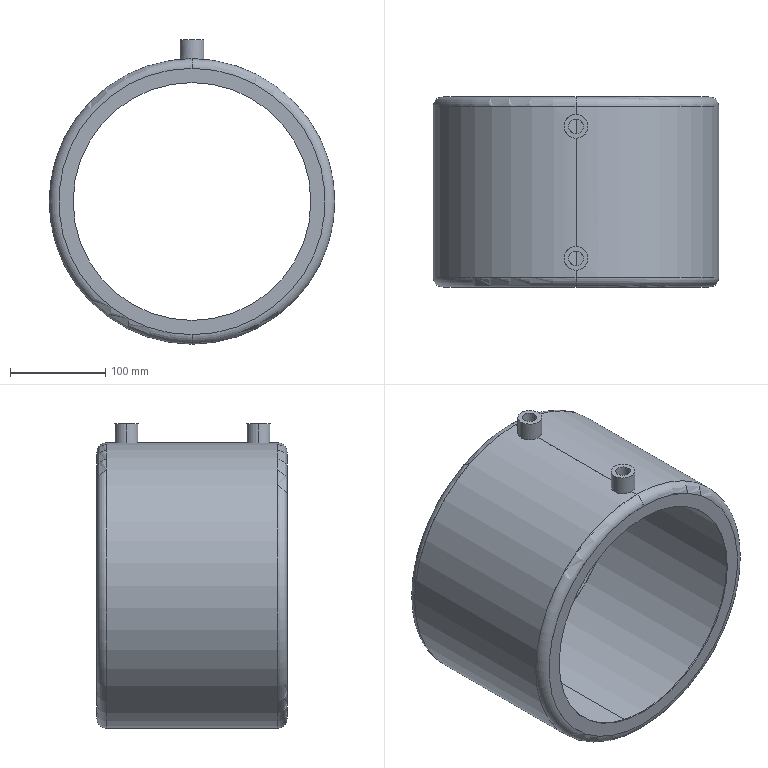Part | SolidWorks | features ICE 2, 3DProfileFeature 1, Extrusion 1, Fillet 1, HoleWzd 1, Shell 1 | 1 solid | 30 faces | box 300 x 200 x 320 mm | volume 277240 mm3 | cylinder 16 | torus 8 | plane 6 | commonest cylinder face diameters 15.25 x4 25 x4 250 x4 297.6 x2 300 x2
STEP:
#1=CARTESIAN_POINT('',(0.,22.375,148.8));
#2=VERTEX_POINT('',#1);
#3=CARTESIAN_POINT('',(-7.625,30.,148.605));
#4=VERTEX_POINT('',#3);
#5=CARTESIAN_POINT('',(0.,22.375,148.8));
#6=CARTESIAN_POINT('',(-0.4973,22.375,148.8));
#7=CARTESIAN_POINT('',(-1.002,22.425,148.797));
#8=CARTESIAN_POINT('',(-1.98,22.62,148.788));
#9=CARTESIAN_POINT('',(-2.455,22.764,148.78));
#10=CARTESIAN_POINT('',(-3.148,23.051,148.767));
#11=CARTESIAN_POINT('',(-3.376,23.159,148.762));
#12=CARTESIAN_POINT('',(-3.818,23.395,148.751));
#13=CARTESIAN_POINT('',(-4.031,23.523,148.746));
#14=CARTESIAN_POINT('',(-4.651,23.937,148.728));
#15=CARTESIAN_POINT('',(-5.036,24.252,148.715));
#16=CARTESIAN_POINT('',(-5.747,24.964,148.689));
#17=CARTESIAN_POINT('',(-6.063,25.35,148.677));
#18=CARTESIAN_POINT('',(-6.477,25.969,148.659));
#19=CARTESIAN_POINT('',(-6.605,26.182,148.653));
#20=CARTESIAN_POINT('',(-6.841,26.623,148.643));
#21=CARTESIAN_POINT('',(-6.949,26.852,148.638));
#22=CARTESIAN_POINT('',(-7.236,27.545,148.624));
#23=CARTESIAN_POINT('',(-7.38,28.02,148.617));
#24=CARTESIAN_POINT('',(-7.575,28.997,148.607));
#25=CARTESIAN_POINT('',(-7.625,29.502,148.605));
#26=CARTESIAN_POINT('',(-7.625,30.,148.605));
#27=B_SPLINE_CURVE_WITH_KNOTS('',3,(#5,#6,#7,#8,#9,#10,#11,#12,#13,#14,#15,#16,#17,#18,#19,#20,#21,#22,#23,#24,#25,#26),.UNSPECIFIED.,.F.,.F.,(4,2,2,2,2,2,2,2,2,2,4),(0.01192,0.01341,0.0149,0.01565,0.01639,0.01788,0.01937,0.02012,0.02086,0.02235,0.02384),.UNSPECIFIED.);
#28=EDGE_CURVE('',#2,#4,#27,.T.);
#29=ORIENTED_EDGE('',*,*,#28,.T.);
#30=CARTESIAN_POINT('',(-7.625,30.,170.));
#31=VERTEX_POINT('',#30);
#32=CARTESIAN_POINT('',(-7.625,30.,170.));
#33=DIRECTION('',(0.,0.,1.));
#34=VECTOR('',#33,1000.);
#35=LINE('',#32,#34);
#36=EDGE_CURVE('',#4,#31,#35,.T.);
#37=ORIENTED_EDGE('',*,*,#36,.T.);
#38=CARTESIAN_POINT('',(7.625,30.,170.));
#39=VERTEX_POINT('',#38);
#40=CARTESIAN_POINT('',(0.,30.,170.));
#41=DIRECTION('',(0.,0.,1.));
#42=DIRECTION('',(1.,0.,0.));
#43=AXIS2_PLACEMENT_3D('',#40,#41,#42);
#44=CIRCLE('',#43,7.625);
#45=EDGE_CURVE('',#31,#39,#44,.T.);
#46=ORIENTED_EDGE('',*,*,#45,.T.);
#47=CARTESIAN_POINT('',(7.625,30.,148.605));
#48=VERTEX_POINT('',#47);
#49=CARTESIAN_POINT('',(7.625,30.,170.));
#50=DIRECTION('',(0.,0.,1.));
#51=VECTOR('',#50,1000.);
#52=LINE('',#49,#51);
#53=EDGE_CURVE('',#48,#39,#52,.T.);
#54=ORIENTED_EDGE('',*,*,#53,.F.);
#55=CARTESIAN_POINT('',(7.625,30.,148.605));
#56=CARTESIAN_POINT('',(7.625,29.496,148.605));
#57=CARTESIAN_POINT('',(7.576,29.,148.607));
#58=CARTESIAN_POINT('',(7.43,28.269,148.614));
#59=CARTESIAN_POINT('',(7.37,28.028,148.617));
#60=CARTESIAN_POINT('',(7.224,27.548,148.625));
#61=CARTESIAN_POINT('',(7.139,27.31,148.629));
#62=CARTESIAN_POINT('',(6.852,26.617,148.642));
#63=CARTESIAN_POINT('',(6.618,26.179,148.653));
#64=CARTESIAN_POINT('',(6.064,25.35,148.677));
#65=CARTESIAN_POINT('',(5.742,24.958,148.69));
#66=CARTESIAN_POINT('',(5.038,24.255,148.715));
#67=CARTESIAN_POINT('',(4.654,23.939,148.728));
#68=CARTESIAN_POINT('',(4.028,23.521,148.746));
#69=CARTESIAN_POINT('',(3.812,23.391,148.751));
#70=CARTESIAN_POINT('',(3.371,23.156,148.762));
#71=CARTESIAN_POINT('',(2.922,22.944,148.772));
#72=CARTESIAN_POINT('',(2.453,22.776,148.78));
#73=CARTESIAN_POINT('',(1.976,22.631,148.787));
#74=CARTESIAN_POINT('',(1.731,22.57,148.79));
#75=CARTESIAN_POINT('',(0.9925,22.423,148.798));
#76=CARTESIAN_POINT('',(0.4975,22.375,148.8));
#77=CARTESIAN_POINT('',(0.,22.375,148.8));
#78=B_SPLINE_CURVE_WITH_KNOTS('',3,(#55,#56,#57,#58,#59,#60,#61,#62,#63,#64,#65,#66,#67,#68,#69,#70,#71,#72,#73,#74,#75,#76,#77),.UNSPECIFIED.,.F.,.F.,(4,2,2,2,2,2,2,2,1,2,2,4),(0.,0.001491,0.002236,0.002981,0.004472,0.005962,0.007453,0.008198,0.008943,0.009688,0.01043,0.01192),.UNSPECIFIED.);
#79=EDGE_CURVE('',#48,#2,#78,.T.);
#80=ORIENTED_EDGE('',*,*,#79,.T.);
#81=EDGE_LOOP('',(#29,#37,#46,#54,#80));
#82=FACE_OUTER_BOUND('',#81,.T.);
#83=CARTESIAN_POINT('',(0.,30.,170.));
#84=DIRECTION('',(0.,0.,1.));
#85=DIRECTION('',(1.,0.,0.));
#86=AXIS2_PLACEMENT_3D('',#83,#84,#85);
#87=CYLINDRICAL_SURFACE('',#86,7.625);
#88=ADVANCED_FACE('',(#82),#87,.F.);
#89=CARTESIAN_POINT('',(0.,161.175,148.8));
#90=VERTEX_POINT('',#89);
#91=CARTESIAN_POINT('',(-7.625,168.8,148.605));
#92=VERTEX_POINT('',#91);
#93=CARTESIAN_POINT('',(0.,161.175,148.8));
#94=CARTESIAN_POINT('',(-0.4973,161.175,148.8));
#95=CARTESIAN_POINT('',(-1.002,161.225,148.797));
#96=CARTESIAN_POINT('',(-1.98,161.42,148.788));
#97=CARTESIAN_POINT('',(-2.455,161.564,148.78));
#98=CARTESIAN_POINT('',(-3.148,161.851,148.767));
#99=CARTESIAN_POINT('',(-3.376,161.959,148.762));
#100=CARTESIAN_POINT('',(-3.818,162.195,148.751));
#101=CARTESIAN_POINT('',(-4.031,162.323,148.746));
#102=CARTESIAN_POINT('',(-4.651,162.737,148.728));
#103=CARTESIAN_POINT('',(-5.036,163.052,148.715));
#104=CARTESIAN_POINT('',(-5.747,163.764,148.689));
#105=CARTESIAN_POINT('',(-6.063,164.15,148.677));
#106=CARTESIAN_POINT('',(-6.477,164.769,148.659));
#107=CARTESIAN_POINT('',(-6.605,164.982,148.653));
#108=CARTESIAN_POINT('',(-6.841,165.423,148.643));
#109=CARTESIAN_POINT('',(-6.949,165.652,148.638));
#110=CARTESIAN_POINT('',(-7.236,166.345,148.624));
#111=CARTESIAN_POINT('',(-7.38,166.82,148.617));
#112=CARTESIAN_POINT('',(-7.575,167.797,148.607));
#113=CARTESIAN_POINT('',(-7.625,168.302,148.605));
#114=CARTESIAN_POINT('',(-7.625,168.8,148.605));
#115=B_SPLINE_CURVE_WITH_KNOTS('',3,(#93,#94,#95,#96,#97,#98,#99,#100,#101,#102,#103,#104,#105,#106,#107,#108,#109,#110,#111,#112,#113,#114),.UNSPECIFIED.,.F.,.F.,(4,2,2,2,2,2,2,2,2,2,4),(0.01192,0.01341,0.0149,0.01565,0.01639,0.01788,0.01937,0.02012,0.02086,0.02235,0.02384),.UNSPECIFIED.);
#116=EDGE_CURVE('',#90,#92,#115,.T.);
#117=ORIENTED_EDGE('',*,*,#116,.T.);
#118=CARTESIAN_POINT('',(-7.625,168.8,170.));
#119=VERTEX_POINT('',#118);
#120=CARTESIAN_POINT('',(-7.625,168.8,170.));
#121=DIRECTION('',(0.,0.,1.));
#122=VECTOR('',#121,1000.);
#123=LINE('',#120,#122);
#124=EDGE_CURVE('',#92,#119,#123,.T.);
#125=ORIENTED_EDGE('',*,*,#124,.T.);
#126=CARTESIAN_POINT('',(7.625,168.8,170.));
#127=VERTEX_POINT('',#126);
#128=CARTESIAN_POINT('',(0.,168.8,170.));
#129=DIRECTION('',(0.,0.,1.));
#130=DIRECTION('',(1.,0.,0.));
#131=AXIS2_PLACEMENT_3D('',#128,#129,#130);
#132=CIRCLE('',#131,7.625);
#133=EDGE_CURVE('',#119,#127,#132,.T.);
#134=ORIENTED_EDGE('',*,*,#133,.T.);
#135=CARTESIAN_POINT('',(7.625,168.8,148.605));
#136=VERTEX_POINT('',#135);
#137=CARTESIAN_POINT('',(7.625,168.8,170.));
#138=DIRECTION('',(0.,0.,1.));
#139=VECTOR('',#138,1000.);
#140=LINE('',#137,#139);
#141=EDGE_CURVE('',#136,#127,#140,.T.);
#142=ORIENTED_EDGE('',*,*,#141,.F.);
#143=CARTESIAN_POINT('',(7.625,168.8,148.605));
#144=CARTESIAN_POINT('',(7.625,168.296,148.605));
#145=CARTESIAN_POINT('',(7.576,167.8,148.607));
#146=CARTESIAN_POINT('',(7.43,167.069,148.614));
#147=CARTESIAN_POINT('',(7.37,166.828,148.617));
#148=CARTESIAN_POINT('',(7.224,166.348,148.625));
#149=CARTESIAN_POINT('',(7.139,166.11,148.629));
#150=CARTESIAN_POINT('',(6.852,165.417,148.642));
#151=CARTESIAN_POINT('',(6.618,164.979,148.653));
#152=CARTESIAN_POINT('',(6.064,164.15,148.677));
#153=CARTESIAN_POINT('',(5.742,163.758,148.69));
#154=CARTESIAN_POINT('',(5.038,163.055,148.715));
#155=CARTESIAN_POINT('',(4.654,162.739,148.728));
#156=CARTESIAN_POINT('',(4.028,162.321,148.746));
#157=CARTESIAN_POINT('',(3.812,162.191,148.751));
#158=CARTESIAN_POINT('',(3.371,161.956,148.762));
#159=CARTESIAN_POINT('',(2.922,161.744,148.772));
#160=CARTESIAN_POINT('',(2.453,161.576,148.78));
#161=CARTESIAN_POINT('',(1.976,161.431,148.787));
#162=CARTESIAN_POINT('',(1.731,161.37,148.79));
#163=CARTESIAN_POINT('',(0.9925,161.223,148.798));
#164=CARTESIAN_POINT('',(0.4975,161.175,148.8));
#165=CARTESIAN_POINT('',(0.,161.175,148.8));
#166=B_SPLINE_CURVE_WITH_KNOTS('',3,(#143,#144,#145,#146,#147,#148,#149,#150,#151,#152,#153,#154,#155,#156,#157,#158,#159,#160,#161,#162,#163,#164,#165),.UNSPECIFIED.,.F.,.F.,(4,2,2,2,2,2,2,2,1,2,2,4),(0.,0.001491,0.002236,0.002981,0.004472,0.005962,0.007453,0.008198,0.008943,0.009688,0.01043,0.01192),.UNSPECIFIED.);
#167=EDGE_CURVE('',#136,#90,#166,.T.);
#168=ORIENTED_EDGE('',*,*,#167,.T.);
#169=EDGE_LOOP('',(#117,#125,#134,#142,#168));
#170=FACE_OUTER_BOUND('',#169,.T.);
#171=CARTESIAN_POINT('',(0.,168.8,170.));
#172=DIRECTION('',(0.,0.,1.));
#173=DIRECTION('',(1.,0.,0.));
#174=AXIS2_PLACEMENT_3D('',#171,#172,#173);
#175=CYLINDRICAL_SURFACE('',#174,7.625);
#176=ADVANCED_FACE('',(#170),#175,.F.);
#177=CARTESIAN_POINT('',(-12.5,168.8,149.478));
#178=VERTEX_POINT('',#177);
#179=CARTESIAN_POINT('',(0.,181.3,150.));
#180=VERTEX_POINT('',#179);
#181=CARTESIAN_POINT('',(-12.5,168.8,149.478));
#182=CARTESIAN_POINT('',(-12.5,169.616,149.478));
#183=CARTESIAN_POINT('',(-12.421,170.428,149.485));
#184=CARTESIAN_POINT('',(-12.181,171.638,149.505));
#185=CARTESIAN_POINT('',(-12.08,172.039,149.513));
#186=CARTESIAN_POINT('',(-11.842,172.823,149.532));
#187=CARTESIAN_POINT('',(-11.567,173.591,149.554));
#188=CARTESIAN_POINT('',(-11.219,174.328,149.58));
#189=CARTESIAN_POINT('',(-10.833,175.049,149.608));
#190=CARTESIAN_POINT('',(-10.621,175.404,149.624));
#191=CARTESIAN_POINT('',(-9.935,176.43,149.671));
#192=CARTESIAN_POINT('',(-9.418,177.06,149.705));
#193=CARTESIAN_POINT('',(-8.553,177.924,149.756));
#194=CARTESIAN_POINT('',(-8.25,178.199,149.773));
#195=CARTESIAN_POINT('',(-7.614,178.722,149.807));
#196=CARTESIAN_POINT('',(-7.282,178.968,149.823));
#197=CARTESIAN_POINT('',(-6.263,179.649,149.871));
#198=CARTESIAN_POINT('',(-5.545,180.033,149.899));
#199=CARTESIAN_POINT('',(-4.41,180.503,149.936));
#200=CARTESIAN_POINT('',(-4.02,180.643,149.947));
#201=CARTESIAN_POINT('',(-3.234,180.881,149.966));
#202=CARTESIAN_POINT('',(-2.837,180.981,149.974));
#203=CARTESIAN_POINT('',(-1.638,181.219,149.993));
#204=CARTESIAN_POINT('',(-0.8258,181.3,150.));
#205=CARTESIAN_POINT('',(0.,181.3,150.));
#206=B_SPLINE_CURVE_WITH_KNOTS('',3,(#181,#182,#183,#184,#185,#186,#187,#188,#189,#190,#191,#192,#193,#194,#195,#196,#197,#198,#199,#200,#201,#202,#203,#204,#205),.UNSPECIFIED.,.F.,.F.,(4,2,2,1,2,2,2,2,2,2,2,2,4),(0.0391,0.04154,0.04276,0.04399,0.04521,0.04643,0.04887,0.0501,0.05132,0.05376,0.05499,0.05621,0.05865),.UNSPECIFIED.);
#207=EDGE_CURVE('',#178,#180,#206,.T.);
#208=ORIENTED_EDGE('',*,*,#207,.F.);
#209=CARTESIAN_POINT('',(-12.5,168.8,170.));
#210=VERTEX_POINT('',#209);
#211=CARTESIAN_POINT('',(-12.5,168.8,-150.001));
#212=DIRECTION('',(0.,0.,1.));
#213=VECTOR('',#212,1000.);
#214=LINE('',#211,#213);
#215=EDGE_CURVE('',#178,#210,#214,.T.);
#216=ORIENTED_EDGE('',*,*,#215,.T.);
#217=CARTESIAN_POINT('',(12.5,168.8,170.));
#218=VERTEX_POINT('',#217);
#219=CARTESIAN_POINT('',(0.,168.8,170.));
#220=DIRECTION('',(0.,0.,1.));
#221=DIRECTION('',(1.,0.,0.));
#222=AXIS2_PLACEMENT_3D('',#219,#220,#221);
#223=CIRCLE('',#222,12.5);
#224=EDGE_CURVE('',#218,#210,#223,.T.);
#225=ORIENTED_EDGE('',*,*,#224,.F.);
#226=CARTESIAN_POINT('',(12.5,168.8,149.478));
#227=VERTEX_POINT('',#226);
#228=CARTESIAN_POINT('',(12.5,168.8,-150.001));
#229=DIRECTION('',(0.,0.,1.));
#230=VECTOR('',#229,1000.);
#231=LINE('',#228,#230);
#232=EDGE_CURVE('',#227,#218,#231,.T.);
#233=ORIENTED_EDGE('',*,*,#232,.F.);
#234=CARTESIAN_POINT('',(0.,181.3,150.));
#235=CARTESIAN_POINT('',(0.8249,181.3,150.));
#236=CARTESIAN_POINT('',(1.639,181.219,149.993));
#237=CARTESIAN_POINT('',(2.836,180.981,149.974));
#238=CARTESIAN_POINT('',(3.232,180.882,149.966));
#239=CARTESIAN_POINT('',(4.016,180.644,149.947));
#240=CARTESIAN_POINT('',(4.407,180.505,149.936));
#241=CARTESIAN_POINT('',(5.542,180.034,149.9));
#242=CARTESIAN_POINT('',(6.259,179.651,149.871));
#243=CARTESIAN_POINT('',(7.278,178.971,149.824));
#244=CARTESIAN_POINT('',(7.608,178.727,149.807));
#245=CARTESIAN_POINT('',(8.245,178.204,149.774));
#246=CARTESIAN_POINT('',(8.548,177.93,149.757));
#247=CARTESIAN_POINT('',(9.412,177.066,149.706));
#248=CARTESIAN_POINT('',(9.93,176.437,149.672));
#249=CARTESIAN_POINT('',(10.615,175.414,149.624));
#250=CARTESIAN_POINT('',(10.828,175.06,149.609));
#251=CARTESIAN_POINT('',(11.214,174.338,149.58));
#252=CARTESIAN_POINT('',(11.562,173.602,149.554));
#253=CARTESIAN_POINT('',(11.838,172.836,149.532));
#254=CARTESIAN_POINT('',(12.076,172.054,149.513));
#255=CARTESIAN_POINT('',(12.177,171.654,149.505));
#256=CARTESIAN_POINT('',(12.419,170.442,149.485));
#257=CARTESIAN_POINT('',(12.5,169.626,149.478));
#258=CARTESIAN_POINT('',(12.5,168.8,149.478));
#259=B_SPLINE_CURVE_WITH_KNOTS('',3,(#234,#235,#236,#237,#238,#239,#240,#241,#242,#243,#244,#245,#246,#247,#248,#249,#250,#251,#252,#253,#254,#255,#256,#257,#258),.UNSPECIFIED.,.F.,.F.,(4,2,2,2,2,2,2,2,2,1,2,2,4),(0.05865,0.06109,0.06231,0.06354,0.06598,0.0672,0.06842,0.07086,0.07208,0.0733,0.07452,0.07574,0.07819),.UNSPECIFIED.);
#260=EDGE_CURVE('',#180,#227,#259,.T.);
#261=ORIENTED_EDGE('',*,*,#260,.F.);
#262=EDGE_LOOP('',(#208,#216,#225,#233,#261));
#263=FACE_OUTER_BOUND('',#262,.T.);
#264=CARTESIAN_POINT('',(0.,168.8,-150.001));
#265=DIRECTION('',(0.,0.,1.));
#266=DIRECTION('',(1.,0.,0.));
#267=AXIS2_PLACEMENT_3D('',#264,#265,#266);
#268=CYLINDRICAL_SURFACE('',#267,12.5);
#269=ADVANCED_FACE('',(#263),#268,.T.);
#270=CARTESIAN_POINT('',(-12.5,30.,149.478));
#271=VERTEX_POINT('',#270);
#272=CARTESIAN_POINT('',(0.,42.5,150.));
#273=VERTEX_POINT('',#272);
#274=CARTESIAN_POINT('',(-12.5,30.,149.478));
#275=CARTESIAN_POINT('',(-12.5,30.816,149.478));
#276=CARTESIAN_POINT('',(-12.421,31.628,149.485));
#277=CARTESIAN_POINT('',(-12.181,32.838,149.505));
#278=CARTESIAN_POINT('',(-12.08,33.239,149.513));
#279=CARTESIAN_POINT('',(-11.842,34.023,149.532));
#280=CARTESIAN_POINT('',(-11.567,34.791,149.554));
#281=CARTESIAN_POINT('',(-11.219,35.528,149.58));
#282=CARTESIAN_POINT('',(-10.833,36.249,149.608));
#283=CARTESIAN_POINT('',(-10.621,36.604,149.624));
#284=CARTESIAN_POINT('',(-9.935,37.63,149.671));
#285=CARTESIAN_POINT('',(-9.418,38.26,149.705));
#286=CARTESIAN_POINT('',(-8.553,39.124,149.756));
#287=CARTESIAN_POINT('',(-8.25,39.399,149.773));
#288=CARTESIAN_POINT('',(-7.614,39.922,149.807));
#289=CARTESIAN_POINT('',(-7.282,40.168,149.823));
#290=CARTESIAN_POINT('',(-6.263,40.849,149.871));
#291=CARTESIAN_POINT('',(-5.545,41.233,149.899));
#292=CARTESIAN_POINT('',(-4.41,41.703,149.936));
#293=CARTESIAN_POINT('',(-4.02,41.843,149.947));
#294=CARTESIAN_POINT('',(-3.234,42.081,149.966));
#295=CARTESIAN_POINT('',(-2.837,42.181,149.974));
#296=CARTESIAN_POINT('',(-1.638,42.419,149.993));
#297=CARTESIAN_POINT('',(-0.8258,42.5,150.));
#298=CARTESIAN_POINT('',(0.,42.5,150.));
#299=B_SPLINE_CURVE_WITH_KNOTS('',3,(#274,#275,#276,#277,#278,#279,#280,#281,#282,#283,#284,#285,#286,#287,#288,#289,#290,#291,#292,#293,#294,#295,#296,#297,#298),.UNSPECIFIED.,.F.,.F.,(4,2,2,1,2,2,2,2,2,2,2,2,4),(0.0391,0.04154,0.04276,0.04399,0.04521,0.04643,0.04887,0.0501,0.05132,0.05376,0.05499,0.05621,0.05865),.UNSPECIFIED.);
#300=EDGE_CURVE('',#271,#273,#299,.T.);
#301=ORIENTED_EDGE('',*,*,#300,.F.);
#302=CARTESIAN_POINT('',(-12.5,30.,170.));
#303=VERTEX_POINT('',#302);
#304=CARTESIAN_POINT('',(-12.5,30.,-150.001));
#305=DIRECTION('',(0.,0.,1.));
#306=VECTOR('',#305,1000.);
#307=LINE('',#304,#306);
#308=EDGE_CURVE('',#271,#303,#307,.T.);
#309=ORIENTED_EDGE('',*,*,#308,.T.);
#310=CARTESIAN_POINT('',(12.5,30.,170.));
#311=VERTEX_POINT('',#310);
#312=CARTESIAN_POINT('',(0.,30.,170.));
#313=DIRECTION('',(0.,0.,1.));
#314=DIRECTION('',(1.,0.,0.));
#315=AXIS2_PLACEMENT_3D('',#312,#313,#314);
#316=CIRCLE('',#315,12.5);
#317=EDGE_CURVE('',#311,#303,#316,.T.);
#318=ORIENTED_EDGE('',*,*,#317,.F.);
#319=CARTESIAN_POINT('',(12.5,30.,149.478));
#320=VERTEX_POINT('',#319);
#321=CARTESIAN_POINT('',(12.5,30.,-150.001));
#322=DIRECTION('',(0.,0.,1.));
#323=VECTOR('',#322,1000.);
#324=LINE('',#321,#323);
#325=EDGE_CURVE('',#320,#311,#324,.T.);
#326=ORIENTED_EDGE('',*,*,#325,.F.);
#327=CARTESIAN_POINT('',(0.,42.5,150.));
#328=CARTESIAN_POINT('',(0.8249,42.5,150.));
#329=CARTESIAN_POINT('',(1.639,42.419,149.993));
#330=CARTESIAN_POINT('',(2.836,42.181,149.974));
#331=CARTESIAN_POINT('',(3.232,42.082,149.966));
#332=CARTESIAN_POINT('',(4.016,41.844,149.947));
#333=CARTESIAN_POINT('',(4.407,41.705,149.936));
#334=CARTESIAN_POINT('',(5.542,41.234,149.9));
#335=CARTESIAN_POINT('',(6.259,40.851,149.871));
#336=CARTESIAN_POINT('',(7.278,40.171,149.824));
#337=CARTESIAN_POINT('',(7.608,39.927,149.807));
#338=CARTESIAN_POINT('',(8.245,39.404,149.774));
#339=CARTESIAN_POINT('',(8.548,39.13,149.757));
#340=CARTESIAN_POINT('',(9.412,38.266,149.706));
#341=CARTESIAN_POINT('',(9.93,37.637,149.672));
#342=CARTESIAN_POINT('',(10.615,36.614,149.624));
#343=CARTESIAN_POINT('',(10.828,36.26,149.609));
#344=CARTESIAN_POINT('',(11.214,35.538,149.58));
#345=CARTESIAN_POINT('',(11.562,34.802,149.554));
#346=CARTESIAN_POINT('',(11.838,34.036,149.532));
#347=CARTESIAN_POINT('',(12.076,33.254,149.513));
#348=CARTESIAN_POINT('',(12.177,32.854,149.505));
#349=CARTESIAN_POINT('',(12.419,31.642,149.485));
#350=CARTESIAN_POINT('',(12.5,30.826,149.478));
#351=CARTESIAN_POINT('',(12.5,30.,149.478));
#352=B_SPLINE_CURVE_WITH_KNOTS('',3,(#327,#328,#329,#330,#331,#332,#333,#334,#335,#336,#337,#338,#339,#340,#341,#342,#343,#344,#345,#346,#347,#348,#349,#350,#351),.UNSPECIFIED.,.F.,.F.,(4,2,2,2,2,2,2,2,2,1,2,2,4),(0.05865,0.06109,0.06231,0.06354,0.06598,0.0672,0.06842,0.07086,0.07208,0.0733,0.07452,0.07574,0.07819),.UNSPECIFIED.);
#353=EDGE_CURVE('',#273,#320,#352,.T.);
#354=ORIENTED_EDGE('',*,*,#353,.F.);
#355=EDGE_LOOP('',(#301,#309,#318,#326,#354));
#356=FACE_OUTER_BOUND('',#355,.T.);
#357=CARTESIAN_POINT('',(0.,30.,-150.001));
#358=DIRECTION('',(0.,0.,1.));
#359=DIRECTION('',(1.,0.,0.));
#360=AXIS2_PLACEMENT_3D('',#357,#358,#359);
#361=CYLINDRICAL_SURFACE('',#360,12.5);
#362=ADVANCED_FACE('',(#356),#361,.T.);
#363=CARTESIAN_POINT('',(0.,190.,148.8));
#364=VERTEX_POINT('',#363);
#365=CARTESIAN_POINT('',(0.,190.,-148.8));
#366=VERTEX_POINT('',#365);
#367=CARTESIAN_POINT('',(0.,190.,0.));
#368=DIRECTION('',(0.,-1.,0.));
#369=DIRECTION('',(0.,0.,-1.));
#370=AXIS2_PLACEMENT_3D('',#367,#368,#369);
#371=CIRCLE('',#370,148.8);
#372=EDGE_CURVE('',#364,#366,#371,.T.);
#373=ORIENTED_EDGE('',*,*,#372,.T.);
#374=CARTESIAN_POINT('',(0.,198.8,-140.));
#375=VERTEX_POINT('',#374);
#376=CARTESIAN_POINT('',(0.,190.,-140.));
#377=DIRECTION('',(1.,0.,0.));
#378=DIRECTION('',(0.,0.,-1.));
#379=AXIS2_PLACEMENT_3D('',#376,#377,#378);
#380=CIRCLE('',#379,8.8);
#381=EDGE_CURVE('',#366,#375,#380,.T.);
#382=ORIENTED_EDGE('',*,*,#381,.T.);
#383=CARTESIAN_POINT('',(0.,198.8,140.));
#384=VERTEX_POINT('',#383);
#385=CARTESIAN_POINT('',(0.,198.8,0.));
#386=DIRECTION('',(0.,1.,0.));
#387=DIRECTION('',(0.,0.,1.));
#388=AXIS2_PLACEMENT_3D('',#385,#386,#387);
#389=CIRCLE('',#388,140.);
#390=EDGE_CURVE('',#375,#384,#389,.T.);
#391=ORIENTED_EDGE('',*,*,#390,.T.);
#392=CARTESIAN_POINT('',(0.,190.,140.));
#393=DIRECTION('',(-1.,0.,0.));
#394=DIRECTION('',(0.,0.,1.));
#395=AXIS2_PLACEMENT_3D('',#392,#393,#394);
#396=CIRCLE('',#395,8.8);
#397=EDGE_CURVE('',#364,#384,#396,.T.);
#398=ORIENTED_EDGE('',*,*,#397,.F.);
#399=EDGE_LOOP('',(#373,#382,#391,#398));
#400=FACE_OUTER_BOUND('',#399,.T.);
#401=CARTESIAN_POINT('',(0.,190.,0.));
#402=DIRECTION('',(0.,1.,0.));
#403=DIRECTION('',(0.,0.,1.));
#404=AXIS2_PLACEMENT_3D('',#401,#402,#403);
#405=TOROIDAL_SURFACE('',#404,140.,8.8);
#406=ADVANCED_FACE('',(#400),#405,.F.);
#407=CARTESIAN_POINT('',(0.,1.2,140.));
#408=VERTEX_POINT('',#407);
#409=CARTESIAN_POINT('',(0.,1.2,-140.));
#410=VERTEX_POINT('',#409);
#411=CARTESIAN_POINT('',(0.,1.2,0.));
#412=DIRECTION('',(0.,-1.,0.));
#413=DIRECTION('',(0.,0.,1.));
#414=AXIS2_PLACEMENT_3D('',#411,#412,#413);
#415=CIRCLE('',#414,140.);
#416=EDGE_CURVE('',#408,#410,#415,.T.);
#417=ORIENTED_EDGE('',*,*,#416,.T.);
#418=CARTESIAN_POINT('',(0.,10.,-148.8));
#419=VERTEX_POINT('',#418);
#420=CARTESIAN_POINT('',(0.,10.,-140.));
#421=DIRECTION('',(1.,0.,0.));
#422=DIRECTION('',(0.,0.,-1.));
#423=AXIS2_PLACEMENT_3D('',#420,#421,#422);
#424=CIRCLE('',#423,8.8);
#425=EDGE_CURVE('',#410,#419,#424,.T.);
#426=ORIENTED_EDGE('',*,*,#425,.T.);
#427=CARTESIAN_POINT('',(0.,10.,148.8));
#428=VERTEX_POINT('',#427);
#429=CARTESIAN_POINT('',(0.,10.,0.));
#430=DIRECTION('',(0.,1.,0.));
#431=DIRECTION('',(0.,0.,-1.));
#432=AXIS2_PLACEMENT_3D('',#429,#430,#431);
#433=CIRCLE('',#432,148.8);
#434=EDGE_CURVE('',#419,#428,#433,.T.);
#435=ORIENTED_EDGE('',*,*,#434,.T.);
#436=CARTESIAN_POINT('',(0.,10.,140.));
#437=DIRECTION('',(-1.,0.,0.));
#438=DIRECTION('',(0.,0.,1.));
#439=AXIS2_PLACEMENT_3D('',#436,#437,#438);
#440=CIRCLE('',#439,8.8);
#441=EDGE_CURVE('',#408,#428,#440,.T.);
#442=ORIENTED_EDGE('',*,*,#441,.F.);
#443=EDGE_LOOP('',(#417,#426,#435,#442));
#444=FACE_OUTER_BOUND('',#443,.T.);
#445=CARTESIAN_POINT('',(0.,10.,0.));
#446=DIRECTION('',(0.,1.,0.));
#447=DIRECTION('',(0.,0.,1.));
#448=AXIS2_PLACEMENT_3D('',#445,#446,#447);
#449=TOROIDAL_SURFACE('',#448,140.,8.8);
#450=ADVANCED_FACE('',(#444),#449,.F.);
#451=ORIENTED_EDGE('',*,*,#372,.F.);
#452=CARTESIAN_POINT('',(0.,176.425,148.8));
#453=VERTEX_POINT('',#452);
#454=CARTESIAN_POINT('',(0.,200.,148.8));
#455=DIRECTION('',(0.,-1.,0.));
#456=VECTOR('',#455,1000.);
#457=LINE('',#454,#456);
#458=EDGE_CURVE('',#364,#453,#457,.T.);
#459=ORIENTED_EDGE('',*,*,#458,.T.);
#460=CARTESIAN_POINT('',(-7.625,168.8,148.605));
#461=CARTESIAN_POINT('',(-7.625,169.298,148.605));
#462=CARTESIAN_POINT('',(-7.577,169.793,148.607));
#463=CARTESIAN_POINT('',(-7.43,170.53,148.614));
#464=CARTESIAN_POINT('',(-7.369,170.776,148.617));
#465=CARTESIAN_POINT('',(-7.224,171.254,148.625));
#466=CARTESIAN_POINT('',(-7.056,171.722,148.633));
#467=CARTESIAN_POINT('',(-6.844,172.172,148.643));
#468=CARTESIAN_POINT('',(-6.609,172.612,148.653));
#469=CARTESIAN_POINT('',(-6.479,172.828,148.659));
#470=CARTESIAN_POINT('',(-6.061,173.454,148.677));
#471=CARTESIAN_POINT('',(-5.745,173.838,148.689));
#472=CARTESIAN_POINT('',(-5.217,174.366,148.709));
#473=CARTESIAN_POINT('',(-5.033,174.534,148.715));
#474=CARTESIAN_POINT('',(-4.645,174.852,148.728));
#475=CARTESIAN_POINT('',(-4.442,175.002,148.734));
#476=CARTESIAN_POINT('',(-3.82,175.418,148.752));
#477=CARTESIAN_POINT('',(-3.382,175.652,148.762));
#478=CARTESIAN_POINT('',(-2.69,175.939,148.776));
#479=CARTESIAN_POINT('',(-2.452,176.024,148.78));
#480=CARTESIAN_POINT('',(-1.972,176.17,148.787));
#481=CARTESIAN_POINT('',(-1.73,176.23,148.79));
#482=CARTESIAN_POINT('',(-0.9986,176.376,148.797));
#483=CARTESIAN_POINT('',(-0.5033,176.425,148.8));
#484=CARTESIAN_POINT('',(0.,176.425,148.8));
#485=B_SPLINE_CURVE_WITH_KNOTS('',3,(#460,#461,#462,#463,#464,#465,#466,#467,#468,#469,#470,#471,#472,#473,#474,#475,#476,#477,#478,#479,#480,#481,#482,#483,#484),.UNSPECIFIED.,.F.,.F.,(4,2,2,1,2,2,2,2,2,2,2,2,4),(0.02384,0.02533,0.02608,0.02682,0.02757,0.02832,0.02981,0.03055,0.0313,0.03279,0.03353,0.03428,0.03577),.UNSPECIFIED.);
#486=EDGE_CURVE('',#92,#453,#485,.T.);
#487=ORIENTED_EDGE('',*,*,#486,.F.);
#488=ORIENTED_EDGE('',*,*,#116,.F.);
#489=CARTESIAN_POINT('',(0.,37.625,148.8));
#490=VERTEX_POINT('',#489);
#491=CARTESIAN_POINT('',(0.,200.,148.8));
#492=DIRECTION('',(0.,-1.,0.));
#493=VECTOR('',#492,1000.);
#494=LINE('',#491,#493);
#495=EDGE_CURVE('',#90,#490,#494,.T.);
#496=ORIENTED_EDGE('',*,*,#495,.T.);
#497=CARTESIAN_POINT('',(-7.625,30.,148.605));
#498=CARTESIAN_POINT('',(-7.625,30.498,148.605));
#499=CARTESIAN_POINT('',(-7.577,30.993,148.607));
#500=CARTESIAN_POINT('',(-7.43,31.73,148.614));
#501=CARTESIAN_POINT('',(-7.369,31.976,148.617));
#502=CARTESIAN_POINT('',(-7.224,32.454,148.625));
#503=CARTESIAN_POINT('',(-7.056,32.922,148.633));
#504=CARTESIAN_POINT('',(-6.844,33.372,148.643));
#505=CARTESIAN_POINT('',(-6.609,33.812,148.653));
#506=CARTESIAN_POINT('',(-6.479,34.028,148.659));
#507=CARTESIAN_POINT('',(-6.061,34.654,148.677));
#508=CARTESIAN_POINT('',(-5.745,35.038,148.689));
#509=CARTESIAN_POINT('',(-5.217,35.566,148.709));
#510=CARTESIAN_POINT('',(-5.033,35.734,148.715));
#511=CARTESIAN_POINT('',(-4.645,36.052,148.728));
#512=CARTESIAN_POINT('',(-4.442,36.202,148.734));
#513=CARTESIAN_POINT('',(-3.82,36.618,148.752));
#514=CARTESIAN_POINT('',(-3.382,36.852,148.762));
#515=CARTESIAN_POINT('',(-2.69,37.139,148.776));
#516=CARTESIAN_POINT('',(-2.452,37.224,148.78));
#517=CARTESIAN_POINT('',(-1.972,37.37,148.787));
#518=CARTESIAN_POINT('',(-1.73,37.43,148.79));
#519=CARTESIAN_POINT('',(-0.9986,37.576,148.797));
#520=CARTESIAN_POINT('',(-0.5033,37.625,148.8));
#521=CARTESIAN_POINT('',(0.,37.625,148.8));
#522=B_SPLINE_CURVE_WITH_KNOTS('',3,(#497,#498,#499,#500,#501,#502,#503,#504,#505,#506,#507,#508,#509,#510,#511,#512,#513,#514,#515,#516,#517,#518,#519,#520,#521),.UNSPECIFIED.,.F.,.F.,(4,2,2,1,2,2,2,2,2,2,2,2,4),(0.02384,0.02533,0.02608,0.02682,0.02757,0.02832,0.02981,0.03055,0.0313,0.03279,0.03353,0.03428,0.03577),.UNSPECIFIED.);
#523=EDGE_CURVE('',#4,#490,#522,.T.);
#524=ORIENTED_EDGE('',*,*,#523,.F.);
#525=ORIENTED_EDGE('',*,*,#28,.F.);
#526=CARTESIAN_POINT('',(0.,200.,148.8));
#527=DIRECTION('',(0.,-1.,0.));
#528=VECTOR('',#527,1000.);
#529=LINE('',#526,#528);
#530=EDGE_CURVE('',#2,#428,#529,.T.);
#531=ORIENTED_EDGE('',*,*,#530,.T.);
#532=ORIENTED_EDGE('',*,*,#434,.F.);
#533=CARTESIAN_POINT('',(0.,200.,-148.8));
#534=DIRECTION('',(0.,-1.,0.));
#535=VECTOR('',#534,1000.);
#536=LINE('',#533,#535);
#537=EDGE_CURVE('',#366,#419,#536,.T.);
#538=ORIENTED_EDGE('',*,*,#537,.F.);
#539=EDGE_LOOP('',(#451,#459,#487,#488,#496,#524,#525,#531,#532,#538));
#540=FACE_OUTER_BOUND('',#539,.T.);
#541=CARTESIAN_POINT('',(0.,200.,0.));
#542=DIRECTION('',(0.,-1.,0.));
#543=DIRECTION('',(0.,0.,-1.));
#544=AXIS2_PLACEMENT_3D('',#541,#542,#543);
#545=CYLINDRICAL_SURFACE('',#544,148.8);
#546=ADVANCED_FACE('',(#540),#545,.F.);
#547=CARTESIAN_POINT('',(0.,0.,-125.));
#548=VERTEX_POINT('',#547);
#549=CARTESIAN_POINT('',(0.,0.,125.));
#550=VERTEX_POINT('',#549);
#551=CARTESIAN_POINT('',(0.,0.,0.));
#552=DIRECTION('',(0.,1.,0.));
#553=DIRECTION('',(0.,0.,1.));
#554=AXIS2_PLACEMENT_3D('',#551,#552,#553);
#555=CIRCLE('',#554,125.);
#556=EDGE_CURVE('',#548,#550,#555,.T.);
#557=ORIENTED_EDGE('',*,*,#556,.F.);
#558=CARTESIAN_POINT('',(0.,1.2,-125.));
#559=VERTEX_POINT('',#558);
#560=CARTESIAN_POINT('',(0.,0.,-125.));
#561=DIRECTION('',(0.,1.,0.));
#562=VECTOR('',#561,1000.);
#563=LINE('',#560,#562);
#564=EDGE_CURVE('',#548,#559,#563,.T.);
#565=ORIENTED_EDGE('',*,*,#564,.T.);
#566=CARTESIAN_POINT('',(0.,1.2,125.));
#567=VERTEX_POINT('',#566);
#568=CARTESIAN_POINT('',(0.,1.2,0.));
#569=DIRECTION('',(0.,1.,0.));
#570=DIRECTION('',(0.,0.,1.));
#571=AXIS2_PLACEMENT_3D('',#568,#569,#570);
#572=CIRCLE('',#571,125.);
#573=EDGE_CURVE('',#559,#567,#572,.T.);
#574=ORIENTED_EDGE('',*,*,#573,.T.);
#575=CARTESIAN_POINT('',(0.,0.,125.));
#576=DIRECTION('',(0.,1.,0.));
#577=VECTOR('',#576,1000.);
#578=LINE('',#575,#577);
#579=EDGE_CURVE('',#550,#567,#578,.T.);
#580=ORIENTED_EDGE('',*,*,#579,.F.);
#581=EDGE_LOOP('',(#557,#565,#574,#580));
#582=FACE_OUTER_BOUND('',#581,.T.);
#583=CARTESIAN_POINT('',(0.,0.,0.));
#584=DIRECTION('',(0.,1.,0.));
#585=DIRECTION('',(0.,0.,1.));
#586=AXIS2_PLACEMENT_3D('',#583,#584,#585);
#587=CYLINDRICAL_SURFACE('',#586,125.);
#588=ADVANCED_FACE('',(#582),#587,.F.);
#589=CARTESIAN_POINT('',(0.,190.,-150.));
#590=VERTEX_POINT('',#589);
#591=CARTESIAN_POINT('',(0.,190.,150.));
#592=VERTEX_POINT('',#591);
#593=CARTESIAN_POINT('',(0.,190.,0.));
#594=DIRECTION('',(0.,-1.,0.));
#595=DIRECTION('',(0.,0.,1.));
#596=AXIS2_PLACEMENT_3D('',#593,#594,#595);
#597=CIRCLE('',#596,150.);
#598=EDGE_CURVE('',#590,#592,#597,.T.);
#599=ORIENTED_EDGE('',*,*,#598,.F.);
#600=CARTESIAN_POINT('',(0.,200.,-140.));
#601=VERTEX_POINT('',#600);
#602=CARTESIAN_POINT('',(0.,190.,-140.));
#603=DIRECTION('',(1.,0.,0.));
#604=DIRECTION('',(0.,0.,-1.));
#605=AXIS2_PLACEMENT_3D('',#602,#603,#604);
#606=CIRCLE('',#605,10.);
#607=EDGE_CURVE('',#590,#601,#606,.T.);
#608=ORIENTED_EDGE('',*,*,#607,.T.);
#609=CARTESIAN_POINT('',(0.,200.,140.));
#610=VERTEX_POINT('',#609);
#611=CARTESIAN_POINT('',(0.,200.,0.));
#612=DIRECTION('',(0.,1.,0.));
#613=DIRECTION('',(0.,0.,1.));
#614=AXIS2_PLACEMENT_3D('',#611,#612,#613);
#615=CIRCLE('',#614,140.);
#616=EDGE_CURVE('',#610,#601,#615,.T.);
#617=ORIENTED_EDGE('',*,*,#616,.F.);
#618=CARTESIAN_POINT('',(0.,190.,140.));
#619=DIRECTION('',(-1.,0.,0.));
#620=DIRECTION('',(0.,0.,1.));
#621=AXIS2_PLACEMENT_3D('',#618,#619,#620);
#622=CIRCLE('',#621,10.);
#623=EDGE_CURVE('',#592,#610,#622,.T.);
#624=ORIENTED_EDGE('',*,*,#623,.F.);
#625=EDGE_LOOP('',(#599,#608,#617,#624));
#626=FACE_OUTER_BOUND('',#625,.T.);
#627=CARTESIAN_POINT('',(0.,190.,0.));
#628=DIRECTION('',(0.,1.,0.));
#629=DIRECTION('',(0.,0.,1.));
#630=AXIS2_PLACEMENT_3D('',#627,#628,#629);
#631=TOROIDAL_SURFACE('',#630,140.,10.);
#632=ADVANCED_FACE('',(#626),#631,.T.);
#633=CARTESIAN_POINT('',(0.,0.,-140.));
#634=VERTEX_POINT('',#633);
#635=CARTESIAN_POINT('',(0.,0.,140.));
#636=VERTEX_POINT('',#635);
#637=CARTESIAN_POINT('',(0.,0.,0.));
#638=DIRECTION('',(0.,-1.,0.));
#639=DIRECTION('',(0.,0.,1.));
#640=AXIS2_PLACEMENT_3D('',#637,#638,#639);
#641=CIRCLE('',#640,140.);
#642=EDGE_CURVE('',#634,#636,#641,.T.);
#643=ORIENTED_EDGE('',*,*,#642,.F.);
#644=CARTESIAN_POINT('',(0.,10.,-150.));
#645=VERTEX_POINT('',#644);
#646=CARTESIAN_POINT('',(0.,10.,-140.));
#647=DIRECTION('',(1.,0.,0.));
#648=DIRECTION('',(0.,0.,-1.));
#649=AXIS2_PLACEMENT_3D('',#646,#647,#648);
#650=CIRCLE('',#649,10.);
#651=EDGE_CURVE('',#634,#645,#650,.T.);
#652=ORIENTED_EDGE('',*,*,#651,.T.);
#653=CARTESIAN_POINT('',(0.,10.,150.));
#654=VERTEX_POINT('',#653);
#655=CARTESIAN_POINT('',(0.,10.,0.));
#656=DIRECTION('',(0.,1.,0.));
#657=DIRECTION('',(0.,0.,1.));
#658=AXIS2_PLACEMENT_3D('',#655,#656,#657);
#659=CIRCLE('',#658,150.);
#660=EDGE_CURVE('',#654,#645,#659,.T.);
#661=ORIENTED_EDGE('',*,*,#660,.F.);
#662=CARTESIAN_POINT('',(0.,10.,140.));
#663=DIRECTION('',(-1.,0.,0.));
#664=DIRECTION('',(0.,0.,1.));
#665=AXIS2_PLACEMENT_3D('',#662,#663,#664);
#666=CIRCLE('',#665,10.);
#667=EDGE_CURVE('',#636,#654,#666,.T.);
#668=ORIENTED_EDGE('',*,*,#667,.F.);
#669=EDGE_LOOP('',(#643,#652,#661,#668));
#670=FACE_OUTER_BOUND('',#669,.T.);
#671=CARTESIAN_POINT('',(0.,10.,0.));
#672=DIRECTION('',(0.,1.,0.));
#673=DIRECTION('',(0.,0.,1.));
#674=AXIS2_PLACEMENT_3D('',#671,#672,#673);
#675=TOROIDAL_SURFACE('',#674,140.,10.);
#676=ADVANCED_FACE('',(#670),#675,.T.);
#677=ORIENTED_EDGE('',*,*,#598,.T.);
#678=CARTESIAN_POINT('',(0.,200.,150.));
#679=DIRECTION('',(0.,-1.,0.));
#680=VECTOR('',#679,1000.);
#681=LINE('',#678,#680);
#682=EDGE_CURVE('',#592,#180,#681,.T.);
#683=ORIENTED_EDGE('',*,*,#682,.T.);
#684=ORIENTED_EDGE('',*,*,#260,.T.);
#685=CARTESIAN_POINT('',(0.,156.3,150.));
#686=VERTEX_POINT('',#685);
#687=CARTESIAN_POINT('',(12.5,168.8,149.478));
#688=CARTESIAN_POINT('',(12.5,167.974,149.478));
#689=CARTESIAN_POINT('',(12.419,167.161,149.485));
#690=CARTESIAN_POINT('',(12.18,165.962,149.505));
#691=CARTESIAN_POINT('',(12.081,165.566,149.513));
#692=CARTESIAN_POINT('',(11.843,164.78,149.532));
#693=CARTESIAN_POINT('',(11.703,164.39,149.543));
#694=CARTESIAN_POINT('',(11.232,163.254,149.579));
#695=CARTESIAN_POINT('',(10.848,162.536,149.608));
#696=CARTESIAN_POINT('',(10.167,161.517,149.655));
#697=CARTESIAN_POINT('',(9.922,161.186,149.672));
#698=CARTESIAN_POINT('',(9.399,160.549,149.705));
#699=CARTESIAN_POINT('',(9.124,160.246,149.723));
#700=CARTESIAN_POINT('',(8.259,159.382,149.774));
#701=CARTESIAN_POINT('',(7.629,158.864,149.807));
#702=CARTESIAN_POINT('',(6.604,158.179,149.855));
#703=CARTESIAN_POINT('',(6.249,157.966,149.87));
#704=CARTESIAN_POINT('',(5.527,157.581,149.899));
#705=CARTESIAN_POINT('',(4.79,157.233,149.925));
#706=CARTESIAN_POINT('',(4.023,156.958,149.947));
#707=CARTESIAN_POINT('',(3.24,156.72,149.966));
#708=CARTESIAN_POINT('',(2.838,156.62,149.974));
#709=CARTESIAN_POINT('',(1.627,156.379,149.993));
#710=CARTESIAN_POINT('',(0.8159,156.3,150.));
#711=CARTESIAN_POINT('',(0.,156.3,150.));
#712=B_SPLINE_CURVE_WITH_KNOTS('',3,(#687,#688,#689,#690,#691,#692,#693,#694,#695,#696,#697,#698,#699,#700,#701,#702,#703,#704,#705,#706,#707,#708,#709,#710,#711),.UNSPECIFIED.,.F.,.F.,(4,2,2,2,2,2,2,2,2,1,2,2,4),(0.,0.002444,0.003666,0.004888,0.007332,0.008555,0.009777,0.01222,0.01344,0.01466,0.01589,0.01711,0.01955),.UNSPECIFIED.);
#713=EDGE_CURVE('',#227,#686,#712,.T.);
#714=ORIENTED_EDGE('',*,*,#713,.T.);
#715=CARTESIAN_POINT('',(0.,200.,150.));
#716=DIRECTION('',(0.,-1.,0.));
#717=VECTOR('',#716,1000.);
#718=LINE('',#715,#717);
#719=EDGE_CURVE('',#686,#273,#718,.T.);
#720=ORIENTED_EDGE('',*,*,#719,.T.);
#721=ORIENTED_EDGE('',*,*,#353,.T.);
#722=CARTESIAN_POINT('',(0.,17.5,150.));
#723=VERTEX_POINT('',#722);
#724=CARTESIAN_POINT('',(12.5,30.,149.478));
#725=CARTESIAN_POINT('',(12.5,29.174,149.478));
#726=CARTESIAN_POINT('',(12.419,28.361,149.485));
#727=CARTESIAN_POINT('',(12.18,27.162,149.505));
#728=CARTESIAN_POINT('',(12.081,26.766,149.513));
#729=CARTESIAN_POINT('',(11.843,25.98,149.532));
#730=CARTESIAN_POINT('',(11.703,25.59,149.543));
#731=CARTESIAN_POINT('',(11.232,24.454,149.579));
#732=CARTESIAN_POINT('',(10.848,23.736,149.608));
#733=CARTESIAN_POINT('',(10.167,22.717,149.655));
#734=CARTESIAN_POINT('',(9.922,22.386,149.672));
#735=CARTESIAN_POINT('',(9.399,21.749,149.705));
#736=CARTESIAN_POINT('',(9.124,21.446,149.723));
#737=CARTESIAN_POINT('',(8.259,20.582,149.774));
#738=CARTESIAN_POINT('',(7.629,20.064,149.807));
#739=CARTESIAN_POINT('',(6.604,19.379,149.855));
#740=CARTESIAN_POINT('',(6.249,19.166,149.87));
#741=CARTESIAN_POINT('',(5.527,18.781,149.899));
#742=CARTESIAN_POINT('',(4.79,18.433,149.925));
#743=CARTESIAN_POINT('',(4.023,18.158,149.947));
#744=CARTESIAN_POINT('',(3.24,17.92,149.966));
#745=CARTESIAN_POINT('',(2.838,17.82,149.974));
#746=CARTESIAN_POINT('',(1.627,17.579,149.993));
#747=CARTESIAN_POINT('',(0.8159,17.5,150.));
#748=CARTESIAN_POINT('',(0.,17.5,150.));
#749=B_SPLINE_CURVE_WITH_KNOTS('',3,(#724,#725,#726,#727,#728,#729,#730,#731,#732,#733,#734,#735,#736,#737,#738,#739,#740,#741,#742,#743,#744,#745,#746,#747,#748),.UNSPECIFIED.,.F.,.F.,(4,2,2,2,2,2,2,2,2,1,2,2,4),(0.,0.002444,0.003666,0.004888,0.007332,0.008555,0.009777,0.01222,0.01344,0.01466,0.01589,0.01711,0.01955),.UNSPECIFIED.);
#750=EDGE_CURVE('',#320,#723,#749,.T.);
#751=ORIENTED_EDGE('',*,*,#750,.T.);
#752=CARTESIAN_POINT('',(0.,200.,150.));
#753=DIRECTION('',(0.,-1.,0.));
#754=VECTOR('',#753,1000.);
#755=LINE('',#752,#754);
#756=EDGE_CURVE('',#723,#654,#755,.T.);
#757=ORIENTED_EDGE('',*,*,#756,.T.);
#758=ORIENTED_EDGE('',*,*,#660,.T.);
#759=CARTESIAN_POINT('',(0.,200.,-150.));
#760=DIRECTION('',(0.,-1.,0.));
#761=VECTOR('',#760,1000.);
#762=LINE('',#759,#761);
#763=EDGE_CURVE('',#590,#645,#762,.T.);
#764=ORIENTED_EDGE('',*,*,#763,.F.);
#765=EDGE_LOOP('',(#677,#683,#684,#714,#720,#721,#751,#757,#758,#764));
#766=FACE_OUTER_BOUND('',#765,.T.);
#767=CARTESIAN_POINT('',(0.,200.,0.));
#768=DIRECTION('',(0.,-1.,0.));
#769=DIRECTION('',(0.,0.,-1.));
#770=AXIS2_PLACEMENT_3D('',#767,#768,#769);
#771=CYLINDRICAL_SURFACE('',#770,150.);
#772=ADVANCED_FACE('',(#766),#771,.T.);
#773=CARTESIAN_POINT('',(0.,198.8,-125.));
#774=VERTEX_POINT('',#773);
#775=CARTESIAN_POINT('',(0.,198.8,125.));
#776=VERTEX_POINT('',#775);
#777=CARTESIAN_POINT('',(0.,198.8,0.));
#778=DIRECTION('',(0.,1.,0.));
#779=DIRECTION('',(0.,0.,1.));
#780=AXIS2_PLACEMENT_3D('',#777,#778,#779);
#781=CIRCLE('',#780,125.);
#782=EDGE_CURVE('',#774,#776,#781,.T.);
#783=ORIENTED_EDGE('',*,*,#782,.F.);
#784=CARTESIAN_POINT('',(0.,200.,-125.));
#785=VERTEX_POINT('',#784);
#786=CARTESIAN_POINT('',(0.,0.,-125.));
#787=DIRECTION('',(0.,1.,0.));
#788=VECTOR('',#787,1000.);
#789=LINE('',#786,#788);
#790=EDGE_CURVE('',#774,#785,#789,.T.);
#791=ORIENTED_EDGE('',*,*,#790,.T.);
#792=CARTESIAN_POINT('',(0.,200.,125.));
#793=VERTEX_POINT('',#792);
#794=CARTESIAN_POINT('',(0.,200.,0.));
#795=DIRECTION('',(0.,1.,0.));
#796=DIRECTION('',(0.,0.,1.));
#797=AXIS2_PLACEMENT_3D('',#794,#795,#796);
#798=CIRCLE('',#797,125.);
#799=EDGE_CURVE('',#785,#793,#798,.T.);
#800=ORIENTED_EDGE('',*,*,#799,.T.);
#801=CARTESIAN_POINT('',(0.,0.,125.));
#802=DIRECTION('',(0.,1.,0.));
#803=VECTOR('',#802,1000.);
#804=LINE('',#801,#803);
#805=EDGE_CURVE('',#776,#793,#804,.T.);
#806=ORIENTED_EDGE('',*,*,#805,.F.);
#807=EDGE_LOOP('',(#783,#791,#800,#806));
#808=FACE_OUTER_BOUND('',#807,.T.);
#809=CARTESIAN_POINT('',(0.,0.,0.));
#810=DIRECTION('',(0.,1.,0.));
#811=DIRECTION('',(0.,0.,1.));
#812=AXIS2_PLACEMENT_3D('',#809,#810,#811);
#813=CYLINDRICAL_SURFACE('',#812,125.);
#814=ADVANCED_FACE('',(#808),#813,.F.);
#815=ORIENTED_EDGE('',*,*,#790,.F.);
#816=CARTESIAN_POINT('',(0.,198.8,0.));
#817=DIRECTION('',(0.,1.,0.));
#818=DIRECTION('',(0.,0.,1.));
#819=AXIS2_PLACEMENT_3D('',#816,#817,#818);
#820=CIRCLE('',#819,125.);
#821=EDGE_CURVE('',#776,#774,#820,.T.);
#822=ORIENTED_EDGE('',*,*,#821,.F.);
#823=ORIENTED_EDGE('',*,*,#805,.T.);
#824=CARTESIAN_POINT('',(0.,200.,0.));
#825=DIRECTION('',(0.,1.,0.));
#826=DIRECTION('',(0.,0.,1.));
#827=AXIS2_PLACEMENT_3D('',#824,#825,#826);
#828=CIRCLE('',#827,125.);
#829=EDGE_CURVE('',#793,#785,#828,.T.);
#830=ORIENTED_EDGE('',*,*,#829,.T.);
#831=EDGE_LOOP('',(#815,#822,#823,#830));
#832=FACE_OUTER_BOUND('',#831,.T.);
#833=CARTESIAN_POINT('',(0.,0.,0.));
#834=DIRECTION('',(0.,1.,0.));
#835=DIRECTION('',(0.,0.,1.));
#836=AXIS2_PLACEMENT_3D('',#833,#834,#835);
#837=CYLINDRICAL_SURFACE('',#836,125.);
#838=ADVANCED_FACE('',(#832),#837,.F.);
#839=ORIENTED_EDGE('',*,*,#682,.F.);
#840=CARTESIAN_POINT('',(0.,190.,0.));
#841=DIRECTION('',(0.,-1.,0.));
#842=DIRECTION('',(0.,0.,1.));
#843=AXIS2_PLACEMENT_3D('',#840,#841,#842);
#844=CIRCLE('',#843,150.);
#845=EDGE_CURVE('',#592,#590,#844,.T.);
#846=ORIENTED_EDGE('',*,*,#845,.T.);
#847=ORIENTED_EDGE('',*,*,#763,.T.);
#848=CARTESIAN_POINT('',(0.,10.,0.));
#849=DIRECTION('',(0.,1.,0.));
#850=DIRECTION('',(0.,0.,1.));
#851=AXIS2_PLACEMENT_3D('',#848,#849,#850);
#852=CIRCLE('',#851,150.);
#853=EDGE_CURVE('',#645,#654,#852,.T.);
#854=ORIENTED_EDGE('',*,*,#853,.T.);
#855=ORIENTED_EDGE('',*,*,#756,.F.);
#856=CARTESIAN_POINT('',(0.,17.5,150.));
#857=CARTESIAN_POINT('',(-0.4078,17.5,150.));
#858=CARTESIAN_POINT('',(-0.8166,17.52,149.998));
#859=CARTESIAN_POINT('',(-1.637,17.601,149.992));
#860=CARTESIAN_POINT('',(-2.045,17.662,149.987));
#861=CARTESIAN_POINT('',(-3.247,17.901,149.967));
#862=CARTESIAN_POINT('',(-4.026,18.138,149.948));
#863=CARTESIAN_POINT('',(-5.161,18.608,149.912));
#864=CARTESIAN_POINT('',(-5.536,18.785,149.898));
#865=CARTESIAN_POINT('',(-6.259,19.172,149.87));
#866=CARTESIAN_POINT('',(-6.609,19.382,149.855));
#867=CARTESIAN_POINT('',(-7.624,20.061,149.808));
#868=CARTESIAN_POINT('',(-8.255,20.578,149.774));
#869=CARTESIAN_POINT('',(-9.422,21.745,149.705));
#870=CARTESIAN_POINT('',(-9.939,22.376,149.671));
#871=CARTESIAN_POINT('',(-10.618,23.391,149.624));
#872=CARTESIAN_POINT('',(-10.828,23.741,149.609));
#873=CARTESIAN_POINT('',(-11.215,24.464,149.58));
#874=CARTESIAN_POINT('',(-11.392,24.839,149.567));
#875=CARTESIAN_POINT('',(-11.862,25.974,149.531));
#876=CARTESIAN_POINT('',(-12.099,26.753,149.511));
#877=CARTESIAN_POINT('',(-12.338,27.955,149.492));
#878=CARTESIAN_POINT('',(-12.399,28.362,149.487));
#879=CARTESIAN_POINT('',(-12.48,29.183,149.48));
#880=CARTESIAN_POINT('',(-12.5,29.592,149.478));
#881=CARTESIAN_POINT('',(-12.5,30.,149.478));
#882=B_SPLINE_CURVE_WITH_KNOTS('',3,(#856,#857,#858,#859,#860,#861,#862,#863,#864,#865,#866,#867,#868,#869,#870,#871,#872,#873,#874,#875,#876,#877,#878,#879,#880,#881),.UNSPECIFIED.,.F.,.F.,(4,2,2,2,2,2,2,2,2,2,2,2,4),(0.01955,0.02077,0.022,0.02444,0.02566,0.02688,0.02933,0.03177,0.03299,0.03421,0.03665,0.03788,0.0391),.UNSPECIFIED.);
#883=EDGE_CURVE('',#723,#271,#882,.T.);
#884=ORIENTED_EDGE('',*,*,#883,.T.);
#885=ORIENTED_EDGE('',*,*,#300,.T.);
#886=ORIENTED_EDGE('',*,*,#719,.F.);
#887=CARTESIAN_POINT('',(0.,156.3,150.));
#888=CARTESIAN_POINT('',(-0.4078,156.3,150.));
#889=CARTESIAN_POINT('',(-0.8166,156.32,149.998));
#890=CARTESIAN_POINT('',(-1.637,156.401,149.992));
#891=CARTESIAN_POINT('',(-2.045,156.462,149.987));
#892=CARTESIAN_POINT('',(-3.247,156.701,149.967));
#893=CARTESIAN_POINT('',(-4.026,156.938,149.948));
#894=CARTESIAN_POINT('',(-5.161,157.408,149.912));
#895=CARTESIAN_POINT('',(-5.536,157.585,149.898));
#896=CARTESIAN_POINT('',(-6.259,157.972,149.87));
#897=CARTESIAN_POINT('',(-6.609,158.182,149.855));
#898=CARTESIAN_POINT('',(-7.624,158.861,149.808));
#899=CARTESIAN_POINT('',(-8.255,159.378,149.774));
#900=CARTESIAN_POINT('',(-9.422,160.545,149.705));
#901=CARTESIAN_POINT('',(-9.939,161.176,149.671));
#902=CARTESIAN_POINT('',(-10.618,162.191,149.624));
#903=CARTESIAN_POINT('',(-10.828,162.541,149.609));
#904=CARTESIAN_POINT('',(-11.215,163.264,149.58));
#905=CARTESIAN_POINT('',(-11.392,163.639,149.567));
#906=CARTESIAN_POINT('',(-11.862,164.774,149.531));
#907=CARTESIAN_POINT('',(-12.099,165.553,149.511));
#908=CARTESIAN_POINT('',(-12.338,166.755,149.492));
#909=CARTESIAN_POINT('',(-12.399,167.162,149.487));
#910=CARTESIAN_POINT('',(-12.48,167.983,149.48));
#911=CARTESIAN_POINT('',(-12.5,168.392,149.478));
#912=CARTESIAN_POINT('',(-12.5,168.8,149.478));
#913=B_SPLINE_CURVE_WITH_KNOTS('',3,(#887,#888,#889,#890,#891,#892,#893,#894,#895,#896,#897,#898,#899,#900,#901,#902,#903,#904,#905,#906,#907,#908,#909,#910,#911,#912),.UNSPECIFIED.,.F.,.F.,(4,2,2,2,2,2,2,2,2,2,2,2,4),(0.01955,0.02077,0.022,0.02444,0.02566,0.02688,0.02933,0.03177,0.03299,0.03421,0.03665,0.03788,0.0391),.UNSPECIFIED.);
#914=EDGE_CURVE('',#686,#178,#913,.T.);
#915=ORIENTED_EDGE('',*,*,#914,.T.);
#916=ORIENTED_EDGE('',*,*,#207,.T.);
#917=EDGE_LOOP('',(#839,#846,#847,#854,#855,#884,#885,#886,#915,#916));
#918=FACE_OUTER_BOUND('',#917,.T.);
#919=CARTESIAN_POINT('',(0.,200.,0.));
#920=DIRECTION('',(0.,-1.,0.));
#921=DIRECTION('',(0.,0.,-1.));
#922=AXIS2_PLACEMENT_3D('',#919,#920,#921);
#923=CYLINDRICAL_SURFACE('',#922,150.);
#924=ADVANCED_FACE('',(#918),#923,.T.);
#925=ORIENTED_EDGE('',*,*,#829,.F.);
#926=ORIENTED_EDGE('',*,*,#799,.F.);
#927=EDGE_LOOP('',(#925,#926));
#928=FACE_BOUND('',#927,.T.);
#929=ORIENTED_EDGE('',*,*,#616,.T.);
#930=CARTESIAN_POINT('',(0.,200.,0.));
#931=DIRECTION('',(0.,1.,0.));
#932=DIRECTION('',(0.,0.,1.));
#933=AXIS2_PLACEMENT_3D('',#930,#931,#932);
#934=CIRCLE('',#933,140.);
#935=EDGE_CURVE('',#601,#610,#934,.T.);
#936=ORIENTED_EDGE('',*,*,#935,.T.);
#937=EDGE_LOOP('',(#929,#936));
#938=FACE_OUTER_BOUND('',#937,.T.);
#939=CARTESIAN_POINT('',(0.,200.,0.));
#940=DIRECTION('',(0.,1.,0.));
#941=DIRECTION('',(0.,0.,1.));
#942=AXIS2_PLACEMENT_3D('',#939,#940,#941);
#943=PLANE('',#942);
#944=ADVANCED_FACE('',(#928,#938),#943,.T.);
#945=CARTESIAN_POINT('',(0.,0.,0.));
#946=DIRECTION('',(0.,1.,0.));
#947=DIRECTION('',(0.,0.,1.));
#948=AXIS2_PLACEMENT_3D('',#945,#946,#947);
#949=CIRCLE('',#948,125.);
#950=EDGE_CURVE('',#550,#548,#949,.T.);
#951=ORIENTED_EDGE('',*,*,#950,.T.);
#952=ORIENTED_EDGE('',*,*,#556,.T.);
#953=EDGE_LOOP('',(#951,#952));
#954=FACE_BOUND('',#953,.T.);
#955=CARTESIAN_POINT('',(0.,0.,0.));
#956=DIRECTION('',(0.,-1.,0.));
#957=DIRECTION('',(0.,0.,1.));
#958=AXIS2_PLACEMENT_3D('',#955,#956,#957);
#959=CIRCLE('',#958,140.);
#960=EDGE_CURVE('',#636,#634,#959,.T.);
#961=ORIENTED_EDGE('',*,*,#960,.T.);
#962=ORIENTED_EDGE('',*,*,#642,.T.);
#963=EDGE_LOOP('',(#961,#962));
#964=FACE_OUTER_BOUND('',#963,.T.);
#965=CARTESIAN_POINT('',(0.,0.,0.));
#966=DIRECTION('',(0.,1.,0.));
#967=DIRECTION('',(0.,0.,1.));
#968=AXIS2_PLACEMENT_3D('',#965,#966,#967);
#969=PLANE('',#968);
#970=ADVANCED_FACE('',(#954,#964),#969,.F.);
#971=ORIENTED_EDGE('',*,*,#651,.F.);
#972=ORIENTED_EDGE('',*,*,#960,.F.);
#973=ORIENTED_EDGE('',*,*,#667,.T.);
#974=ORIENTED_EDGE('',*,*,#853,.F.);
#975=EDGE_LOOP('',(#971,#972,#973,#974));
#976=FACE_OUTER_BOUND('',#975,.T.);
#977=CARTESIAN_POINT('',(0.,10.,0.));
#978=DIRECTION('',(0.,1.,0.));
#979=DIRECTION('',(0.,0.,1.));
#980=AXIS2_PLACEMENT_3D('',#977,#978,#979);
#981=TOROIDAL_SURFACE('',#980,140.,10.);
#982=ADVANCED_FACE('',(#976),#981,.T.);
#983=ORIENTED_EDGE('',*,*,#607,.F.);
#984=ORIENTED_EDGE('',*,*,#845,.F.);
#985=ORIENTED_EDGE('',*,*,#623,.T.);
#986=ORIENTED_EDGE('',*,*,#935,.F.);
#987=EDGE_LOOP('',(#983,#984,#985,#986));
#988=FACE_OUTER_BOUND('',#987,.T.);
#989=CARTESIAN_POINT('',(0.,190.,0.));
#990=DIRECTION('',(0.,1.,0.));
#991=DIRECTION('',(0.,0.,1.));
#992=AXIS2_PLACEMENT_3D('',#989,#990,#991);
#993=TOROIDAL_SURFACE('',#992,140.,10.);
#994=ADVANCED_FACE('',(#988),#993,.T.);
#995=ORIENTED_EDGE('',*,*,#564,.F.);
#996=ORIENTED_EDGE('',*,*,#950,.F.);
#997=ORIENTED_EDGE('',*,*,#579,.T.);
#998=CARTESIAN_POINT('',(0.,1.2,0.));
#999=DIRECTION('',(0.,1.,0.));
#1000=DIRECTION('',(0.,0.,1.));
#1001=AXIS2_PLACEMENT_3D('',#998,#999,#1000);
#1002=CIRCLE('',#1001,125.);
#1003=EDGE_CURVE('',#567,#559,#1002,.T.);
#1004=ORIENTED_EDGE('',*,*,#1003,.T.);
#1005=EDGE_LOOP('',(#995,#996,#997,#1004));
#1006=FACE_OUTER_BOUND('',#1005,.T.);
#1007=CARTESIAN_POINT('',(0.,0.,0.));
#1008=DIRECTION('',(0.,1.,0.));
#1009=DIRECTION('',(0.,0.,1.));
#1010=AXIS2_PLACEMENT_3D('',#1007,#1008,#1009);
#1011=CYLINDRICAL_SURFACE('',#1010,125.);
#1012=ADVANCED_FACE('',(#1006),#1011,.F.);
#1013=ORIENTED_EDGE('',*,*,#458,.F.);
#1014=CARTESIAN_POINT('',(0.,190.,0.));
#1015=DIRECTION('',(0.,-1.,0.));
#1016=DIRECTION('',(0.,0.,-1.));
#1017=AXIS2_PLACEMENT_3D('',#1014,#1015,#1016);
#1018=CIRCLE('',#1017,148.8);
#1019=EDGE_CURVE('',#366,#364,#1018,.T.);
#1020=ORIENTED_EDGE('',*,*,#1019,.F.);
#1021=ORIENTED_EDGE('',*,*,#537,.T.);
#1022=CARTESIAN_POINT('',(0.,10.,0.));
#1023=DIRECTION('',(0.,1.,0.));
#1024=DIRECTION('',(0.,0.,-1.));
#1025=AXIS2_PLACEMENT_3D('',#1022,#1023,#1024);
#1026=CIRCLE('',#1025,148.8);
#1027=EDGE_CURVE('',#428,#419,#1026,.T.);
#1028=ORIENTED_EDGE('',*,*,#1027,.F.);
#1029=ORIENTED_EDGE('',*,*,#530,.F.);
#1030=ORIENTED_EDGE('',*,*,#79,.F.);
#1031=CARTESIAN_POINT('',(0.,37.625,148.8));
#1032=CARTESIAN_POINT('',(0.5028,37.625,148.8));
#1033=CARTESIAN_POINT('',(0.9996,37.575,148.797));
#1034=CARTESIAN_POINT('',(1.73,37.43,148.79));
#1035=CARTESIAN_POINT('',(1.971,37.37,148.787));
#1036=CARTESIAN_POINT('',(2.45,37.225,148.78));
#1037=CARTESIAN_POINT('',(2.688,37.14,148.776));
#1038=CARTESIAN_POINT('',(3.38,36.853,148.762));
#1039=CARTESIAN_POINT('',(3.818,36.619,148.752));
#1040=CARTESIAN_POINT('',(4.646,36.067,148.728));
#1041=CARTESIAN_POINT('',(5.038,35.745,148.715));
#1042=CARTESIAN_POINT('',(5.742,35.042,148.69));
#1043=CARTESIAN_POINT('',(6.057,34.658,148.677));
#1044=CARTESIAN_POINT('',(6.475,34.035,148.659));
#1045=CARTESIAN_POINT('',(6.605,33.818,148.653));
#1046=CARTESIAN_POINT('',(6.84,33.378,148.643));
#1047=CARTESIAN_POINT('',(6.947,33.153,148.638));
#1048=CARTESIAN_POINT('',(7.232,32.466,148.624));
#1049=CARTESIAN_POINT('',(7.379,31.988,148.617));
#1050=CARTESIAN_POINT('',(7.576,31.002,148.607));
#1051=CARTESIAN_POINT('',(7.625,30.504,148.605));
#1052=CARTESIAN_POINT('',(7.625,30.,148.605));
#1053=B_SPLINE_CURVE_WITH_KNOTS('',3,(#1031,#1032,#1033,#1034,#1035,#1036,#1037,#1038,#1039,#1040,#1041,#1042,#1043,#1044,#1045,#1046,#1047,#1048,#1049,#1050,#1051,#1052),.UNSPECIFIED.,.F.,.F.,(4,2,2,2,2,2,2,2,2,2,4),(0.03577,0.03726,0.038,0.03875,0.04024,0.04172,0.04321,0.04396,0.0447,0.04619,0.04768),.UNSPECIFIED.);
#1054=EDGE_CURVE('',#490,#48,#1053,.T.);
#1055=ORIENTED_EDGE('',*,*,#1054,.F.);
#1056=ORIENTED_EDGE('',*,*,#495,.F.);
#1057=ORIENTED_EDGE('',*,*,#167,.F.);
#1058=CARTESIAN_POINT('',(0.,176.425,148.8));
#1059=CARTESIAN_POINT('',(0.5028,176.425,148.8));
#1060=CARTESIAN_POINT('',(0.9996,176.375,148.797));
#1061=CARTESIAN_POINT('',(1.73,176.23,148.79));
#1062=CARTESIAN_POINT('',(1.971,176.17,148.787));
#1063=CARTESIAN_POINT('',(2.45,176.025,148.78));
#1064=CARTESIAN_POINT('',(2.688,175.94,148.776));
#1065=CARTESIAN_POINT('',(3.38,175.653,148.762));
#1066=CARTESIAN_POINT('',(3.818,175.419,148.752));
#1067=CARTESIAN_POINT('',(4.646,174.867,148.728));
#1068=CARTESIAN_POINT('',(5.038,174.545,148.715));
#1069=CARTESIAN_POINT('',(5.742,173.842,148.69));
#1070=CARTESIAN_POINT('',(6.057,173.458,148.677));
#1071=CARTESIAN_POINT('',(6.475,172.835,148.659));
#1072=CARTESIAN_POINT('',(6.605,172.618,148.653));
#1073=CARTESIAN_POINT('',(6.84,172.178,148.643));
#1074=CARTESIAN_POINT('',(6.947,171.953,148.638));
#1075=CARTESIAN_POINT('',(7.232,171.266,148.624));
#1076=CARTESIAN_POINT('',(7.379,170.788,148.617));
#1077=CARTESIAN_POINT('',(7.576,169.802,148.607));
#1078=CARTESIAN_POINT('',(7.625,169.304,148.605));
#1079=CARTESIAN_POINT('',(7.625,168.8,148.605));
#1080=B_SPLINE_CURVE_WITH_KNOTS('',3,(#1058,#1059,#1060,#1061,#1062,#1063,#1064,#1065,#1066,#1067,#1068,#1069,#1070,#1071,#1072,#1073,#1074,#1075,#1076,#1077,#1078,#1079),.UNSPECIFIED.,.F.,.F.,(4,2,2,2,2,2,2,2,2,2,4),(0.03577,0.03726,0.038,0.03875,0.04024,0.04172,0.04321,0.04396,0.0447,0.04619,0.04768),.UNSPECIFIED.);
#1081=EDGE_CURVE('',#453,#136,#1080,.T.);
#1082=ORIENTED_EDGE('',*,*,#1081,.F.);
#1083=EDGE_LOOP('',(#1013,#1020,#1021,#1028,#1029,#1030,#1055,#1056,#1057,#1082));
#1084=FACE_OUTER_BOUND('',#1083,.T.);
#1085=CARTESIAN_POINT('',(0.,200.,0.));
#1086=DIRECTION('',(0.,-1.,0.));
#1087=DIRECTION('',(0.,0.,-1.));
#1088=AXIS2_PLACEMENT_3D('',#1085,#1086,#1087);
#1089=CYLINDRICAL_SURFACE('',#1088,148.8);
#1090=ADVANCED_FACE('',(#1084),#1089,.F.);
#1091=ORIENTED_EDGE('',*,*,#821,.T.);
#1092=ORIENTED_EDGE('',*,*,#782,.T.);
#1093=EDGE_LOOP('',(#1091,#1092));
#1094=FACE_BOUND('',#1093,.T.);
#1095=CARTESIAN_POINT('',(0.,198.8,0.));
#1096=DIRECTION('',(0.,1.,0.));
#1097=DIRECTION('',(0.,0.,1.));
#1098=AXIS2_PLACEMENT_3D('',#1095,#1096,#1097);
#1099=CIRCLE('',#1098,140.);
#1100=EDGE_CURVE('',#384,#375,#1099,.T.);
#1101=ORIENTED_EDGE('',*,*,#1100,.F.);
#1102=ORIENTED_EDGE('',*,*,#390,.F.);
#1103=EDGE_LOOP('',(#1101,#1102));
#1104=FACE_OUTER_BOUND('',#1103,.T.);
#1105=CARTESIAN_POINT('',(0.,198.8,0.));
#1106=DIRECTION('',(0.,1.,0.));
#1107=DIRECTION('',(0.,0.,1.));
#1108=AXIS2_PLACEMENT_3D('',#1105,#1106,#1107);
#1109=PLANE('',#1108);
#1110=ADVANCED_FACE('',(#1094,#1104),#1109,.F.);
#1111=ORIENTED_EDGE('',*,*,#1003,.F.);
#1112=ORIENTED_EDGE('',*,*,#573,.F.);
#1113=EDGE_LOOP('',(#1111,#1112));
#1114=FACE_BOUND('',#1113,.T.);
#1115=ORIENTED_EDGE('',*,*,#416,.F.);
#1116=CARTESIAN_POINT('',(0.,1.2,0.));
#1117=DIRECTION('',(0.,-1.,0.));
#1118=DIRECTION('',(0.,0.,1.));
#1119=AXIS2_PLACEMENT_3D('',#1116,#1117,#1118);
#1120=CIRCLE('',#1119,140.);
#1121=EDGE_CURVE('',#410,#408,#1120,.T.);
#1122=ORIENTED_EDGE('',*,*,#1121,.F.);
#1123=EDGE_LOOP('',(#1115,#1122));
#1124=FACE_OUTER_BOUND('',#1123,.T.);
#1125=CARTESIAN_POINT('',(0.,1.2,0.));
#1126=DIRECTION('',(0.,1.,0.));
#1127=DIRECTION('',(0.,0.,1.));
#1128=AXIS2_PLACEMENT_3D('',#1125,#1126,#1127);
#1129=PLANE('',#1128);
#1130=ADVANCED_FACE('',(#1114,#1124),#1129,.T.);
#1131=ORIENTED_EDGE('',*,*,#425,.F.);
#1132=ORIENTED_EDGE('',*,*,#1121,.T.);
#1133=ORIENTED_EDGE('',*,*,#441,.T.);
#1134=ORIENTED_EDGE('',*,*,#1027,.T.);
#1135=EDGE_LOOP('',(#1131,#1132,#1133,#1134));
#1136=FACE_OUTER_BOUND('',#1135,.T.);
#1137=CARTESIAN_POINT('',(0.,10.,0.));
#1138=DIRECTION('',(0.,1.,0.));
#1139=DIRECTION('',(0.,0.,1.));
#1140=AXIS2_PLACEMENT_3D('',#1137,#1138,#1139);
#1141=TOROIDAL_SURFACE('',#1140,140.,8.8);
#1142=ADVANCED_FACE('',(#1136),#1141,.F.);
#1143=ORIENTED_EDGE('',*,*,#381,.F.);
#1144=ORIENTED_EDGE('',*,*,#1019,.T.);
#1145=ORIENTED_EDGE('',*,*,#397,.T.);
#1146=ORIENTED_EDGE('',*,*,#1100,.T.);
#1147=EDGE_LOOP('',(#1143,#1144,#1145,#1146));
#1148=FACE_OUTER_BOUND('',#1147,.T.);
#1149=CARTESIAN_POINT('',(0.,190.,0.));
#1150=DIRECTION('',(0.,1.,0.));
#1151=DIRECTION('',(0.,0.,1.));
#1152=AXIS2_PLACEMENT_3D('',#1149,#1150,#1151);
#1153=TOROIDAL_SURFACE('',#1152,140.,8.8);
#1154=ADVANCED_FACE('',(#1148),#1153,.F.);
#1155=ORIENTED_EDGE('',*,*,#308,.F.);
#1156=ORIENTED_EDGE('',*,*,#883,.F.);
#1157=ORIENTED_EDGE('',*,*,#750,.F.);
#1158=ORIENTED_EDGE('',*,*,#325,.T.);
#1159=CARTESIAN_POINT('',(0.,30.,170.));
#1160=DIRECTION('',(0.,0.,1.));
#1161=DIRECTION('',(1.,0.,0.));
#1162=AXIS2_PLACEMENT_3D('',#1159,#1160,#1161);
#1163=CIRCLE('',#1162,12.5);
#1164=EDGE_CURVE('',#303,#311,#1163,.T.);
#1165=ORIENTED_EDGE('',*,*,#1164,.F.);
#1166=EDGE_LOOP('',(#1155,#1156,#1157,#1158,#1165));
#1167=FACE_OUTER_BOUND('',#1166,.T.);
#1168=CARTESIAN_POINT('',(0.,30.,-150.001));
#1169=DIRECTION('',(0.,0.,1.));
#1170=DIRECTION('',(1.,0.,0.));
#1171=AXIS2_PLACEMENT_3D('',#1168,#1169,#1170);
#1172=CYLINDRICAL_SURFACE('',#1171,12.5);
#1173=ADVANCED_FACE('',(#1167),#1172,.T.);
#1174=CARTESIAN_POINT('',(0.,30.,170.));
#1175=DIRECTION('',(0.,0.,1.));
#1176=DIRECTION('',(1.,0.,0.));
#1177=AXIS2_PLACEMENT_3D('',#1174,#1175,#1176);
#1178=CIRCLE('',#1177,7.625);
#1179=EDGE_CURVE('',#39,#31,#1178,.T.);
#1180=ORIENTED_EDGE('',*,*,#1179,.F.);
#1181=ORIENTED_EDGE('',*,*,#45,.F.);
#1182=EDGE_LOOP('',(#1180,#1181));
#1183=FACE_BOUND('',#1182,.T.);
#1184=ORIENTED_EDGE('',*,*,#317,.T.);
#1185=ORIENTED_EDGE('',*,*,#1164,.T.);
#1186=EDGE_LOOP('',(#1184,#1185));
#1187=FACE_OUTER_BOUND('',#1186,.T.);
#1188=CARTESIAN_POINT('',(0.,30.,170.));
#1189=DIRECTION('',(0.,0.,1.));
#1190=DIRECTION('',(1.,0.,0.));
#1191=AXIS2_PLACEMENT_3D('',#1188,#1189,#1190);
#1192=PLANE('',#1191);
#1193=ADVANCED_FACE('',(#1183,#1187),#1192,.T.);
#1194=ORIENTED_EDGE('',*,*,#215,.F.);
#1195=ORIENTED_EDGE('',*,*,#914,.F.);
#1196=ORIENTED_EDGE('',*,*,#713,.F.);
#1197=ORIENTED_EDGE('',*,*,#232,.T.);
#1198=CARTESIAN_POINT('',(0.,168.8,170.));
#1199=DIRECTION('',(0.,0.,1.));
#1200=DIRECTION('',(1.,0.,0.));
#1201=AXIS2_PLACEMENT_3D('',#1198,#1199,#1200);
#1202=CIRCLE('',#1201,12.5);
#1203=EDGE_CURVE('',#210,#218,#1202,.T.);
#1204=ORIENTED_EDGE('',*,*,#1203,.F.);
#1205=EDGE_LOOP('',(#1194,#1195,#1196,#1197,#1204));
#1206=FACE_OUTER_BOUND('',#1205,.T.);
#1207=CARTESIAN_POINT('',(0.,168.8,-150.001));
#1208=DIRECTION('',(0.,0.,1.));
#1209=DIRECTION('',(1.,0.,0.));
#1210=AXIS2_PLACEMENT_3D('',#1207,#1208,#1209);
#1211=CYLINDRICAL_SURFACE('',#1210,12.5);
#1212=ADVANCED_FACE('',(#1206),#1211,.T.);
#1213=CARTESIAN_POINT('',(0.,168.8,170.));
#1214=DIRECTION('',(0.,0.,1.));
#1215=DIRECTION('',(1.,0.,0.));
#1216=AXIS2_PLACEMENT_3D('',#1213,#1214,#1215);
#1217=CIRCLE('',#1216,7.625);
#1218=EDGE_CURVE('',#127,#119,#1217,.T.);
#1219=ORIENTED_EDGE('',*,*,#1218,.F.);
#1220=ORIENTED_EDGE('',*,*,#133,.F.);
#1221=EDGE_LOOP('',(#1219,#1220));
#1222=FACE_BOUND('',#1221,.T.);
#1223=ORIENTED_EDGE('',*,*,#224,.T.);
#1224=ORIENTED_EDGE('',*,*,#1203,.T.);
#1225=EDGE_LOOP('',(#1223,#1224));
#1226=FACE_OUTER_BOUND('',#1225,.T.);
#1227=CARTESIAN_POINT('',(0.,168.8,170.));
#1228=DIRECTION('',(0.,0.,1.));
#1229=DIRECTION('',(1.,0.,0.));
#1230=AXIS2_PLACEMENT_3D('',#1227,#1228,#1229);
#1231=PLANE('',#1230);
#1232=ADVANCED_FACE('',(#1222,#1226),#1231,.T.);
#1233=ORIENTED_EDGE('',*,*,#124,.F.);
#1234=ORIENTED_EDGE('',*,*,#486,.T.);
#1235=ORIENTED_EDGE('',*,*,#1081,.T.);
#1236=ORIENTED_EDGE('',*,*,#141,.T.);
#1237=ORIENTED_EDGE('',*,*,#1218,.T.);
#1238=EDGE_LOOP('',(#1233,#1234,#1235,#1236,#1237));
#1239=FACE_OUTER_BOUND('',#1238,.T.);
#1240=CARTESIAN_POINT('',(0.,168.8,170.));
#1241=DIRECTION('',(0.,0.,1.));
#1242=DIRECTION('',(1.,0.,0.));
#1243=AXIS2_PLACEMENT_3D('',#1240,#1241,#1242);
#1244=CYLINDRICAL_SURFACE('',#1243,7.625);
#1245=ADVANCED_FACE('',(#1239),#1244,.F.);
#1246=ORIENTED_EDGE('',*,*,#36,.F.);
#1247=ORIENTED_EDGE('',*,*,#523,.T.);
#1248=ORIENTED_EDGE('',*,*,#1054,.T.);
#1249=ORIENTED_EDGE('',*,*,#53,.T.);
#1250=ORIENTED_EDGE('',*,*,#1179,.T.);
#1251=EDGE_LOOP('',(#1246,#1247,#1248,#1249,#1250));
#1252=FACE_OUTER_BOUND('',#1251,.T.);
#1253=CARTESIAN_POINT('',(0.,30.,170.));
#1254=DIRECTION('',(0.,0.,1.));
#1255=DIRECTION('',(1.,0.,0.));
#1256=AXIS2_PLACEMENT_3D('',#1253,#1254,#1255);
#1257=CYLINDRICAL_SURFACE('',#1256,7.625);
#1258=ADVANCED_FACE('',(#1252),#1257,.F.);
#1259=CLOSED_SHELL('',(#88,#176,#269,#362,#406,#450,#546,#588,#632,#676,#772,#814,#838,#924,#944,#970,#982,#994,#1012,#1090,#1110,#1130,#1142,#1154,#1173,#1193,#1212,#1232,#1245,#1258));
#1260=MANIFOLD_SOLID_BREP('',#1259);
#1261=CARTESIAN_POINT('',(0.,0.,0.));
#1262=DIRECTION('',(0.,0.,1.));
#1263=DIRECTION('',(1.,0.,0.));
#1264=AXIS2_PLACEMENT_3D('',#1261,#1262,#1263);
#1265=(LENGTH_UNIT()NAMED_UNIT(*)SI_UNIT(.MILLI.,.METRE.));
#1266=UNCERTAINTY_MEASURE_WITH_UNIT(LENGTH_MEASURE(0.00001),#1265,'','');
#1267=(NAMED_UNIT(*)PLANE_ANGLE_UNIT()SI_UNIT($,.RADIAN.));
#1268=(NAMED_UNIT(*)SI_UNIT($,.STERADIAN.)SOLID_ANGLE_UNIT());
#1269=(GEOMETRIC_REPRESENTATION_CONTEXT(3)GLOBAL_UNCERTAINTY_ASSIGNED_CONTEXT((#1266))GLOBAL_UNIT_ASSIGNED_CONTEXT((#1265,#1267,#1268))REPRESENTATION_CONTEXT('',''));
#1270=ADVANCED_BREP_SHAPE_REPRESENTATION('',(#1260,#1264),#1269);